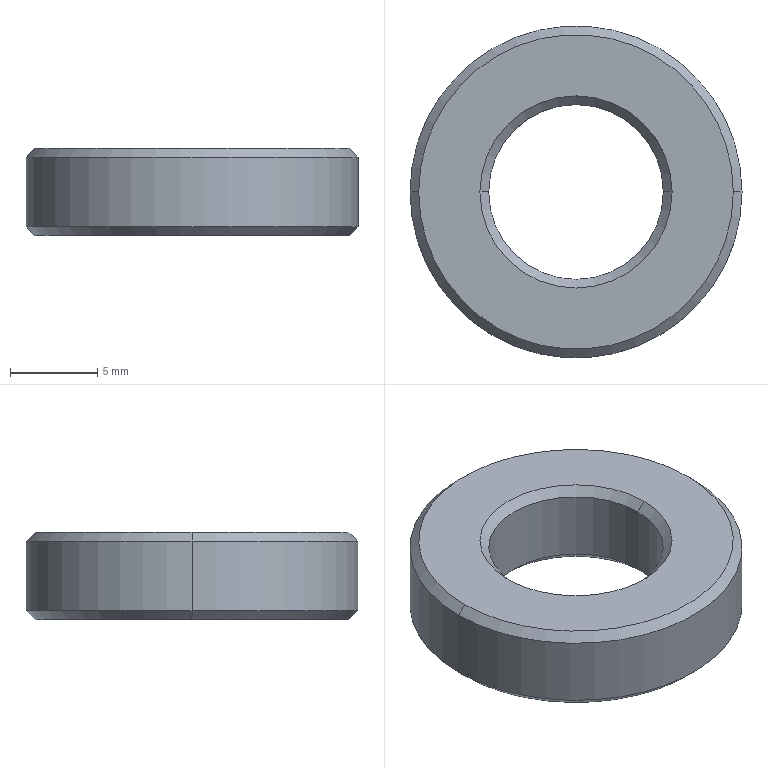Part | STEP file | deep groove bearing 6800 | 1 solid | 14 faces | box 19 x 19 x 5 mm | volume 1002 mm3 | cone 8 | cylinder 4 | plane 2 | commonest cylinder face diameters 10 x2 19 x2
STEP:
#1=CARTESIAN_POINT('',(0.,0.,0.));
#2=DIRECTION('',(0.,0.,1.));
#3=DIRECTION('',(1.,0.,0.));
#4=AXIS2_PLACEMENT_3D('',#1,#2,#3);
#5=CARTESIAN_POINT('',(9.,0.,5.));
#6=VERTEX_POINT('',#5);
#7=CARTESIAN_POINT('',(-9.,0.,5.));
#8=VERTEX_POINT('',#7);
#9=CARTESIAN_POINT('',(0.,0.,5.));
#10=DIRECTION('',(0.,0.,1.));
#11=DIRECTION('',(1.,0.,0.));
#12=AXIS2_PLACEMENT_3D('',#9,#10,#11);
#13=CIRCLE('',#12,9.);
#14=CARTESIAN_POINT('',(0.,0.,5.));
#15=DIRECTION('',(0.,0.,-1.));
#16=DIRECTION('',(-1.,0.,0.));
#17=AXIS2_PLACEMENT_3D('',#14,#15,#16);
#18=CONICAL_SURFACE('',#17,9.,0.7854);
#19=CARTESIAN_POINT('',(3.142,0.));
#20=DIRECTION('',(-1.,0.));
#21=VECTOR('',#20,1.);
#22=LINE('',#19,#21);
#23=(GEOMETRIC_REPRESENTATION_CONTEXT(2)PARAMETRIC_REPRESENTATION_CONTEXT()REPRESENTATION_CONTEXT('',''));
#24=DEFINITIONAL_REPRESENTATION('',(#22),#23);
#25=PCURVE('',#18,#24);
#26=CARTESIAN_POINT('',(0.,0.,5.));
#27=DIRECTION('',(0.,0.,1.));
#28=DIRECTION('',(1.,0.,0.));
#29=AXIS2_PLACEMENT_3D('',#26,#27,#28);
#30=PLANE('',#29);
#31=CARTESIAN_POINT('',(0.,0.));
#32=DIRECTION('',(1.,0.));
#33=AXIS2_PLACEMENT_2D('',#31,#32);
#34=CIRCLE('',#33,9.);
#35=(GEOMETRIC_REPRESENTATION_CONTEXT(2)PARAMETRIC_REPRESENTATION_CONTEXT()REPRESENTATION_CONTEXT('',''));
#36=DEFINITIONAL_REPRESENTATION('',(#34),#35);
#37=PCURVE('',#30,#36);
#38=SURFACE_CURVE('',#13,(#25,#37),.PCURVE_S1.);
#39=EDGE_CURVE('',#6,#8,#38,.T.);
#40=ORIENTED_EDGE('',*,*,#39,.F.);
#41=CARTESIAN_POINT('',(9.5,0.,4.5));
#42=VERTEX_POINT('',#41);
#43=CARTESIAN_POINT('',(9.,0.,5.));
#44=DIRECTION('',(0.7071,0.,-0.7071));
#45=VECTOR('',#44,1.);
#46=LINE('',#43,#45);
#47=CARTESIAN_POINT('',(3.142,0.));
#48=DIRECTION('',(0.,1.));
#49=VECTOR('',#48,1.);
#50=LINE('',#47,#49);
#51=(GEOMETRIC_REPRESENTATION_CONTEXT(2)PARAMETRIC_REPRESENTATION_CONTEXT()REPRESENTATION_CONTEXT('',''));
#52=DEFINITIONAL_REPRESENTATION('',(#50),#51);
#53=PCURVE('',#18,#52);
#54=CARTESIAN_POINT('',(0.,0.,5.));
#55=DIRECTION('',(0.,0.,-1.));
#56=DIRECTION('',(-1.,0.,0.));
#57=AXIS2_PLACEMENT_3D('',#54,#55,#56);
#58=CONICAL_SURFACE('',#57,9.,0.7854);
#59=CARTESIAN_POINT('',(3.142,0.));
#60=DIRECTION('',(0.,1.));
#61=VECTOR('',#60,1.);
#62=LINE('',#59,#61);
#63=(GEOMETRIC_REPRESENTATION_CONTEXT(2)PARAMETRIC_REPRESENTATION_CONTEXT()REPRESENTATION_CONTEXT('',''));
#64=DEFINITIONAL_REPRESENTATION('',(#62),#63);
#65=PCURVE('',#58,#64);
#66=SURFACE_CURVE('',#46,(#53,#65),.PCURVE_S1.);
#67=EDGE_CURVE('',#6,#42,#66,.T.);
#68=ORIENTED_EDGE('',*,*,#67,.T.);
#69=CARTESIAN_POINT('',(-9.5,0.,4.5));
#70=VERTEX_POINT('',#69);
#71=CARTESIAN_POINT('',(0.,0.,4.5));
#72=DIRECTION('',(0.,0.,-1.));
#73=DIRECTION('',(1.,0.,0.));
#74=AXIS2_PLACEMENT_3D('',#71,#72,#73);
#75=CIRCLE('',#74,9.5);
#76=CARTESIAN_POINT('',(-3.142,0.5));
#77=DIRECTION('',(1.,0.));
#78=VECTOR('',#77,1.);
#79=LINE('',#76,#78);
#80=(GEOMETRIC_REPRESENTATION_CONTEXT(2)PARAMETRIC_REPRESENTATION_CONTEXT()REPRESENTATION_CONTEXT('',''));
#81=DEFINITIONAL_REPRESENTATION('',(#79),#80);
#82=PCURVE('',#18,#81);
#83=CARTESIAN_POINT('',(0.,0.,5.));
#84=DIRECTION('',(0.,0.,-1.));
#85=DIRECTION('',(-1.,0.,0.));
#86=AXIS2_PLACEMENT_3D('',#83,#84,#85);
#87=CYLINDRICAL_SURFACE('',#86,9.5);
#88=CARTESIAN_POINT('',(-3.142,0.5));
#89=DIRECTION('',(1.,0.));
#90=VECTOR('',#89,1.);
#91=LINE('',#88,#90);
#92=(GEOMETRIC_REPRESENTATION_CONTEXT(2)PARAMETRIC_REPRESENTATION_CONTEXT()REPRESENTATION_CONTEXT('',''));
#93=DEFINITIONAL_REPRESENTATION('',(#91),#92);
#94=PCURVE('',#87,#93);
#95=SURFACE_CURVE('',#75,(#82,#94),.PCURVE_S1.);
#96=EDGE_CURVE('',#70,#42,#95,.T.);
#97=ORIENTED_EDGE('',*,*,#96,.F.);
#98=CARTESIAN_POINT('',(-9.,0.,5.));
#99=DIRECTION('',(-0.7071,0.,-0.7071));
#100=VECTOR('',#99,1.);
#101=LINE('',#98,#100);
#102=CARTESIAN_POINT('',(0.,0.));
#103=DIRECTION('',(0.,1.));
#104=VECTOR('',#103,1.);
#105=LINE('',#102,#104);
#106=(GEOMETRIC_REPRESENTATION_CONTEXT(2)PARAMETRIC_REPRESENTATION_CONTEXT()REPRESENTATION_CONTEXT('',''));
#107=DEFINITIONAL_REPRESENTATION('',(#105),#106);
#108=PCURVE('',#18,#107);
#109=CARTESIAN_POINT('',(6.283,0.));
#110=DIRECTION('',(0.,1.));
#111=VECTOR('',#110,1.);
#112=LINE('',#109,#111);
#113=(GEOMETRIC_REPRESENTATION_CONTEXT(2)PARAMETRIC_REPRESENTATION_CONTEXT()REPRESENTATION_CONTEXT('',''));
#114=DEFINITIONAL_REPRESENTATION('',(#112),#113);
#115=PCURVE('',#58,#114);
#116=SURFACE_CURVE('',#101,(#108,#115),.PCURVE_S1.);
#117=EDGE_CURVE('',#8,#70,#116,.T.);
#118=ORIENTED_EDGE('',*,*,#117,.F.);
#119=EDGE_LOOP('',(#40,#68,#97,#118));
#120=FACE_BOUND('',#119,.T.);
#121=ADVANCED_FACE('',(#120),#18,.T.);
#122=CARTESIAN_POINT('',(-9.,0.,0.));
#123=VERTEX_POINT('',#122);
#124=CARTESIAN_POINT('',(9.,0.,0.));
#125=VERTEX_POINT('',#124);
#126=CARTESIAN_POINT('',(0.,0.,0.));
#127=DIRECTION('',(0.,0.,-1.));
#128=DIRECTION('',(1.,0.,0.));
#129=AXIS2_PLACEMENT_3D('',#126,#127,#128);
#130=CIRCLE('',#129,9.);
#131=CARTESIAN_POINT('',(0.,0.,0.5));
#132=DIRECTION('',(0.,0.,1.));
#133=DIRECTION('',(1.,0.,0.));
#134=AXIS2_PLACEMENT_3D('',#131,#132,#133);
#135=CONICAL_SURFACE('',#134,9.5,0.7854);
#136=CARTESIAN_POINT('',(6.283,-0.5));
#137=DIRECTION('',(-1.,0.));
#138=VECTOR('',#137,1.);
#139=LINE('',#136,#138);
#140=(GEOMETRIC_REPRESENTATION_CONTEXT(2)PARAMETRIC_REPRESENTATION_CONTEXT()REPRESENTATION_CONTEXT('',''));
#141=DEFINITIONAL_REPRESENTATION('',(#139),#140);
#142=PCURVE('',#135,#141);
#143=CARTESIAN_POINT('',(0.,0.,0.));
#144=DIRECTION('',(0.,0.,1.));
#145=DIRECTION('',(1.,0.,0.));
#146=AXIS2_PLACEMENT_3D('',#143,#144,#145);
#147=PLANE('',#146);
#148=CARTESIAN_POINT('',(9.,0.));
#149=CARTESIAN_POINT('',(9.,-15.588));
#150=CARTESIAN_POINT('',(-4.5,-7.794));
#151=CARTESIAN_POINT('',(-18.,0.));
#152=CARTESIAN_POINT('',(-4.5,7.794));
#153=CARTESIAN_POINT('',(9.,15.588));
#154=CARTESIAN_POINT('',(9.,0.));
#155=(BOUNDED_CURVE()B_SPLINE_CURVE(2,(#148,#149,#150,#151,#152,#153,#154),.UNSPECIFIED.,.T.,.F.)B_SPLINE_CURVE_WITH_KNOTS((1,2,2,2,2,1),(-2.094,0.,2.094,4.189,6.283,8.378),.UNSPECIFIED.)CURVE()GEOMETRIC_REPRESENTATION_ITEM()RATIONAL_B_SPLINE_CURVE((1.,0.5,1.,0.5,1.,0.5,1.))REPRESENTATION_ITEM(''));
#156=(GEOMETRIC_REPRESENTATION_CONTEXT(2)PARAMETRIC_REPRESENTATION_CONTEXT()REPRESENTATION_CONTEXT('',''));
#157=DEFINITIONAL_REPRESENTATION('',(#155),#156);
#158=PCURVE('',#147,#157);
#159=SURFACE_CURVE('',#130,(#142,#158),.PCURVE_S1.);
#160=EDGE_CURVE('',#123,#125,#159,.T.);
#161=ORIENTED_EDGE('',*,*,#160,.F.);
#162=CARTESIAN_POINT('',(-9.5,0.,0.5));
#163=VERTEX_POINT('',#162);
#164=CARTESIAN_POINT('',(-9.5,0.,0.5));
#165=DIRECTION('',(-0.7071,0.,0.7071));
#166=VECTOR('',#165,1.);
#167=LINE('',#164,#166);
#168=CARTESIAN_POINT('',(3.142,0.));
#169=DIRECTION('',(0.,1.));
#170=VECTOR('',#169,1.);
#171=LINE('',#168,#170);
#172=(GEOMETRIC_REPRESENTATION_CONTEXT(2)PARAMETRIC_REPRESENTATION_CONTEXT()REPRESENTATION_CONTEXT('',''));
#173=DEFINITIONAL_REPRESENTATION('',(#171),#172);
#174=PCURVE('',#135,#173);
#175=CARTESIAN_POINT('',(0.,0.,0.5));
#176=DIRECTION('',(0.,0.,1.));
#177=DIRECTION('',(1.,0.,0.));
#178=AXIS2_PLACEMENT_3D('',#175,#176,#177);
#179=CONICAL_SURFACE('',#178,9.5,0.7854);
#180=CARTESIAN_POINT('',(3.142,0.));
#181=DIRECTION('',(0.,1.));
#182=VECTOR('',#181,1.);
#183=LINE('',#180,#182);
#184=(GEOMETRIC_REPRESENTATION_CONTEXT(2)PARAMETRIC_REPRESENTATION_CONTEXT()REPRESENTATION_CONTEXT('',''));
#185=DEFINITIONAL_REPRESENTATION('',(#183),#184);
#186=PCURVE('',#179,#185);
#187=SURFACE_CURVE('',#167,(#174,#186),.PCURVE_S1.);
#188=EDGE_CURVE('',#123,#163,#187,.T.);
#189=ORIENTED_EDGE('',*,*,#188,.T.);
#190=CARTESIAN_POINT('',(9.5,0.,0.5));
#191=VERTEX_POINT('',#190);
#192=CARTESIAN_POINT('',(0.,0.,0.5));
#193=DIRECTION('',(0.,0.,1.));
#194=DIRECTION('',(1.,0.,0.));
#195=AXIS2_PLACEMENT_3D('',#192,#193,#194);
#196=CIRCLE('',#195,9.5);
#197=CARTESIAN_POINT('',(0.,0.));
#198=DIRECTION('',(1.,0.));
#199=VECTOR('',#198,1.);
#200=LINE('',#197,#199);
#201=(GEOMETRIC_REPRESENTATION_CONTEXT(2)PARAMETRIC_REPRESENTATION_CONTEXT()REPRESENTATION_CONTEXT('',''));
#202=DEFINITIONAL_REPRESENTATION('',(#200),#201);
#203=PCURVE('',#135,#202);
#204=CARTESIAN_POINT('',(3.142,4.5));
#205=DIRECTION('',(-1.,0.));
#206=VECTOR('',#205,1.);
#207=LINE('',#204,#206);
#208=(GEOMETRIC_REPRESENTATION_CONTEXT(2)PARAMETRIC_REPRESENTATION_CONTEXT()REPRESENTATION_CONTEXT('',''));
#209=DEFINITIONAL_REPRESENTATION('',(#207),#208);
#210=PCURVE('',#87,#209);
#211=SURFACE_CURVE('',#196,(#203,#210),.PCURVE_S1.);
#212=EDGE_CURVE('',#191,#163,#211,.T.);
#213=ORIENTED_EDGE('',*,*,#212,.F.);
#214=CARTESIAN_POINT('',(9.5,0.,0.5));
#215=DIRECTION('',(0.7071,0.,0.7071));
#216=VECTOR('',#215,1.);
#217=LINE('',#214,#216);
#218=CARTESIAN_POINT('',(0.,0.));
#219=DIRECTION('',(0.,1.));
#220=VECTOR('',#219,1.);
#221=LINE('',#218,#220);
#222=(GEOMETRIC_REPRESENTATION_CONTEXT(2)PARAMETRIC_REPRESENTATION_CONTEXT()REPRESENTATION_CONTEXT('',''));
#223=DEFINITIONAL_REPRESENTATION('',(#221),#222);
#224=PCURVE('',#135,#223);
#225=CARTESIAN_POINT('',(6.283,0.));
#226=DIRECTION('',(0.,1.));
#227=VECTOR('',#226,1.);
#228=LINE('',#225,#227);
#229=(GEOMETRIC_REPRESENTATION_CONTEXT(2)PARAMETRIC_REPRESENTATION_CONTEXT()REPRESENTATION_CONTEXT('',''));
#230=DEFINITIONAL_REPRESENTATION('',(#228),#229);
#231=PCURVE('',#179,#230);
#232=SURFACE_CURVE('',#217,(#224,#231),.PCURVE_S1.);
#233=EDGE_CURVE('',#125,#191,#232,.T.);
#234=ORIENTED_EDGE('',*,*,#233,.F.);
#235=EDGE_LOOP('',(#161,#189,#213,#234));
#236=FACE_BOUND('',#235,.T.);
#237=ADVANCED_FACE('',(#236),#135,.T.);
#238=CARTESIAN_POINT('',(5.,0.,4.5));
#239=VERTEX_POINT('',#238);
#240=CARTESIAN_POINT('',(5.5,0.,5.));
#241=VERTEX_POINT('',#240);
#242=CARTESIAN_POINT('',(5.,0.,4.5));
#243=DIRECTION('',(0.7071,0.,0.7071));
#244=VECTOR('',#243,1.);
#245=LINE('',#242,#244);
#246=CARTESIAN_POINT('',(0.,0.,4.5));
#247=DIRECTION('',(0.,0.,1.));
#248=DIRECTION('',(1.,0.,0.));
#249=AXIS2_PLACEMENT_3D('',#246,#247,#248);
#250=CONICAL_SURFACE('',#249,5.,0.7854);
#251=CARTESIAN_POINT('',(6.283,0.));
#252=DIRECTION('',(0.,1.));
#253=VECTOR('',#252,1.);
#254=LINE('',#251,#253);
#255=(GEOMETRIC_REPRESENTATION_CONTEXT(2)PARAMETRIC_REPRESENTATION_CONTEXT()REPRESENTATION_CONTEXT('',''));
#256=DEFINITIONAL_REPRESENTATION('',(#254),#255);
#257=PCURVE('',#250,#256);
#258=CARTESIAN_POINT('',(0.,0.,4.5));
#259=DIRECTION('',(0.,0.,1.));
#260=DIRECTION('',(1.,0.,0.));
#261=AXIS2_PLACEMENT_3D('',#258,#259,#260);
#262=CONICAL_SURFACE('',#261,5.,0.7854);
#263=CARTESIAN_POINT('',(0.,0.));
#264=DIRECTION('',(0.,1.));
#265=VECTOR('',#264,1.);
#266=LINE('',#263,#265);
#267=(GEOMETRIC_REPRESENTATION_CONTEXT(2)PARAMETRIC_REPRESENTATION_CONTEXT()REPRESENTATION_CONTEXT('',''));
#268=DEFINITIONAL_REPRESENTATION('',(#266),#267);
#269=PCURVE('',#262,#268);
#270=SURFACE_CURVE('',#245,(#257,#269),.PCURVE_S1.);
#271=EDGE_CURVE('',#239,#241,#270,.T.);
#272=ORIENTED_EDGE('',*,*,#271,.T.);
#273=CARTESIAN_POINT('',(-5.5,0.,5.));
#274=VERTEX_POINT('',#273);
#275=CARTESIAN_POINT('',(0.,0.,5.));
#276=DIRECTION('',(0.,0.,-1.));
#277=DIRECTION('',(1.,0.,0.));
#278=AXIS2_PLACEMENT_3D('',#275,#276,#277);
#279=CIRCLE('',#278,5.5);
#280=CARTESIAN_POINT('',(6.283,0.5));
#281=DIRECTION('',(-1.,0.));
#282=VECTOR('',#281,1.);
#283=LINE('',#280,#282);
#284=(GEOMETRIC_REPRESENTATION_CONTEXT(2)PARAMETRIC_REPRESENTATION_CONTEXT()REPRESENTATION_CONTEXT('',''));
#285=DEFINITIONAL_REPRESENTATION('',(#283),#284);
#286=PCURVE('',#250,#285);
#287=CARTESIAN_POINT('',(5.5,0.));
#288=CARTESIAN_POINT('',(5.5,-9.526));
#289=CARTESIAN_POINT('',(-2.75,-4.763));
#290=CARTESIAN_POINT('',(-11.,0.));
#291=CARTESIAN_POINT('',(-2.75,4.763));
#292=CARTESIAN_POINT('',(5.5,9.526));
#293=CARTESIAN_POINT('',(5.5,0.));
#294=(BOUNDED_CURVE()B_SPLINE_CURVE(2,(#287,#288,#289,#290,#291,#292,#293),.UNSPECIFIED.,.T.,.F.)B_SPLINE_CURVE_WITH_KNOTS((1,2,2,2,2,1),(-2.094,0.,2.094,4.189,6.283,8.378),.UNSPECIFIED.)CURVE()GEOMETRIC_REPRESENTATION_ITEM()RATIONAL_B_SPLINE_CURVE((1.,0.5,1.,0.5,1.,0.5,1.))REPRESENTATION_ITEM(''));
#295=(GEOMETRIC_REPRESENTATION_CONTEXT(2)PARAMETRIC_REPRESENTATION_CONTEXT()REPRESENTATION_CONTEXT('',''));
#296=DEFINITIONAL_REPRESENTATION('',(#294),#295);
#297=PCURVE('',#30,#296);
#298=SURFACE_CURVE('',#279,(#286,#297),.PCURVE_S1.);
#299=EDGE_CURVE('',#241,#274,#298,.T.);
#300=ORIENTED_EDGE('',*,*,#299,.T.);
#301=CARTESIAN_POINT('',(-5.,0.,4.5));
#302=VERTEX_POINT('',#301);
#303=CARTESIAN_POINT('',(-5.,0.,4.5));
#304=DIRECTION('',(-0.7071,0.,0.7071));
#305=VECTOR('',#304,1.);
#306=LINE('',#303,#305);
#307=CARTESIAN_POINT('',(3.142,0.));
#308=DIRECTION('',(0.,1.));
#309=VECTOR('',#308,1.);
#310=LINE('',#307,#309);
#311=(GEOMETRIC_REPRESENTATION_CONTEXT(2)PARAMETRIC_REPRESENTATION_CONTEXT()REPRESENTATION_CONTEXT('',''));
#312=DEFINITIONAL_REPRESENTATION('',(#310),#311);
#313=PCURVE('',#250,#312);
#314=CARTESIAN_POINT('',(3.142,0.));
#315=DIRECTION('',(0.,1.));
#316=VECTOR('',#315,1.);
#317=LINE('',#314,#316);
#318=(GEOMETRIC_REPRESENTATION_CONTEXT(2)PARAMETRIC_REPRESENTATION_CONTEXT()REPRESENTATION_CONTEXT('',''));
#319=DEFINITIONAL_REPRESENTATION('',(#317),#318);
#320=PCURVE('',#262,#319);
#321=SURFACE_CURVE('',#306,(#313,#320),.PCURVE_S1.);
#322=EDGE_CURVE('',#302,#274,#321,.T.);
#323=ORIENTED_EDGE('',*,*,#322,.F.);
#324=CARTESIAN_POINT('',(0.,0.,4.5));
#325=DIRECTION('',(0.,0.,1.));
#326=DIRECTION('',(1.,0.,0.));
#327=AXIS2_PLACEMENT_3D('',#324,#325,#326);
#328=CIRCLE('',#327,5.);
#329=CARTESIAN_POINT('',(0.,0.));
#330=DIRECTION('',(1.,0.));
#331=VECTOR('',#330,1.);
#332=LINE('',#329,#331);
#333=(GEOMETRIC_REPRESENTATION_CONTEXT(2)PARAMETRIC_REPRESENTATION_CONTEXT()REPRESENTATION_CONTEXT('',''));
#334=DEFINITIONAL_REPRESENTATION('',(#332),#333);
#335=PCURVE('',#250,#334);
#336=CARTESIAN_POINT('',(0.,0.,5.));
#337=DIRECTION('',(0.,0.,-1.));
#338=DIRECTION('',(-1.,0.,0.));
#339=AXIS2_PLACEMENT_3D('',#336,#337,#338);
#340=CYLINDRICAL_SURFACE('',#339,5.);
#341=CARTESIAN_POINT('',(9.425,0.5));
#342=DIRECTION('',(-1.,0.));
#343=VECTOR('',#342,1.);
#344=LINE('',#341,#343);
#345=(GEOMETRIC_REPRESENTATION_CONTEXT(2)PARAMETRIC_REPRESENTATION_CONTEXT()REPRESENTATION_CONTEXT('',''));
#346=DEFINITIONAL_REPRESENTATION('',(#344),#345);
#347=PCURVE('',#340,#346);
#348=SURFACE_CURVE('',#328,(#335,#347),.PCURVE_S1.);
#349=EDGE_CURVE('',#302,#239,#348,.T.);
#350=ORIENTED_EDGE('',*,*,#349,.T.);
#351=EDGE_LOOP('',(#272,#300,#323,#350));
#352=FACE_BOUND('',#351,.F.);
#353=ADVANCED_FACE('',(#352),#250,.F.);
#354=CARTESIAN_POINT('',(-5.,0.,0.5));
#355=VERTEX_POINT('',#354);
#356=CARTESIAN_POINT('',(-5.5,0.,0.));
#357=VERTEX_POINT('',#356);
#358=CARTESIAN_POINT('',(-5.5,0.,0.));
#359=DIRECTION('',(-0.7071,0.,-0.7071));
#360=VECTOR('',#359,1.);
#361=LINE('',#358,#360);
#362=CARTESIAN_POINT('',(0.,0.,0.));
#363=DIRECTION('',(0.,0.,-1.));
#364=DIRECTION('',(-1.,0.,0.));
#365=AXIS2_PLACEMENT_3D('',#362,#363,#364);
#366=CONICAL_SURFACE('',#365,5.5,0.7854);
#367=CARTESIAN_POINT('',(6.283,0.));
#368=DIRECTION('',(0.,1.));
#369=VECTOR('',#368,1.);
#370=LINE('',#367,#369);
#371=(GEOMETRIC_REPRESENTATION_CONTEXT(2)PARAMETRIC_REPRESENTATION_CONTEXT()REPRESENTATION_CONTEXT('',''));
#372=DEFINITIONAL_REPRESENTATION('',(#370),#371);
#373=PCURVE('',#366,#372);
#374=CARTESIAN_POINT('',(0.,0.,0.));
#375=DIRECTION('',(0.,0.,-1.));
#376=DIRECTION('',(-1.,0.,0.));
#377=AXIS2_PLACEMENT_3D('',#374,#375,#376);
#378=CONICAL_SURFACE('',#377,5.5,0.7854);
#379=CARTESIAN_POINT('',(0.,0.));
#380=DIRECTION('',(0.,1.));
#381=VECTOR('',#380,1.);
#382=LINE('',#379,#381);
#383=(GEOMETRIC_REPRESENTATION_CONTEXT(2)PARAMETRIC_REPRESENTATION_CONTEXT()REPRESENTATION_CONTEXT('',''));
#384=DEFINITIONAL_REPRESENTATION('',(#382),#383);
#385=PCURVE('',#378,#384);
#386=SURFACE_CURVE('',#361,(#373,#385),.PCURVE_S1.);
#387=EDGE_CURVE('',#355,#357,#386,.T.);
#388=ORIENTED_EDGE('',*,*,#387,.T.);
#389=CARTESIAN_POINT('',(5.5,0.,0.));
#390=VERTEX_POINT('',#389);
#391=CARTESIAN_POINT('',(0.,0.,0.));
#392=DIRECTION('',(0.,0.,1.));
#393=DIRECTION('',(1.,0.,0.));
#394=AXIS2_PLACEMENT_3D('',#391,#392,#393);
#395=CIRCLE('',#394,5.5);
#396=CARTESIAN_POINT('',(9.425,0.));
#397=DIRECTION('',(-1.,0.));
#398=VECTOR('',#397,1.);
#399=LINE('',#396,#398);
#400=(GEOMETRIC_REPRESENTATION_CONTEXT(2)PARAMETRIC_REPRESENTATION_CONTEXT()REPRESENTATION_CONTEXT('',''));
#401=DEFINITIONAL_REPRESENTATION('',(#399),#400);
#402=PCURVE('',#366,#401);
#403=CARTESIAN_POINT('',(0.,0.));
#404=DIRECTION('',(1.,0.));
#405=AXIS2_PLACEMENT_2D('',#403,#404);
#406=CIRCLE('',#405,5.5);
#407=(GEOMETRIC_REPRESENTATION_CONTEXT(2)PARAMETRIC_REPRESENTATION_CONTEXT()REPRESENTATION_CONTEXT('',''));
#408=DEFINITIONAL_REPRESENTATION('',(#406),#407);
#409=PCURVE('',#147,#408);
#410=SURFACE_CURVE('',#395,(#402,#409),.PCURVE_S1.);
#411=EDGE_CURVE('',#357,#390,#410,.T.);
#412=ORIENTED_EDGE('',*,*,#411,.T.);
#413=CARTESIAN_POINT('',(5.,0.,0.5));
#414=VERTEX_POINT('',#413);
#415=CARTESIAN_POINT('',(5.5,0.,0.));
#416=DIRECTION('',(0.7071,0.,-0.7071));
#417=VECTOR('',#416,1.);
#418=LINE('',#415,#417);
#419=CARTESIAN_POINT('',(3.142,0.));
#420=DIRECTION('',(0.,1.));
#421=VECTOR('',#420,1.);
#422=LINE('',#419,#421);
#423=(GEOMETRIC_REPRESENTATION_CONTEXT(2)PARAMETRIC_REPRESENTATION_CONTEXT()REPRESENTATION_CONTEXT('',''));
#424=DEFINITIONAL_REPRESENTATION('',(#422),#423);
#425=PCURVE('',#366,#424);
#426=CARTESIAN_POINT('',(3.142,0.));
#427=DIRECTION('',(0.,1.));
#428=VECTOR('',#427,1.);
#429=LINE('',#426,#428);
#430=(GEOMETRIC_REPRESENTATION_CONTEXT(2)PARAMETRIC_REPRESENTATION_CONTEXT()REPRESENTATION_CONTEXT('',''));
#431=DEFINITIONAL_REPRESENTATION('',(#429),#430);
#432=PCURVE('',#378,#431);
#433=SURFACE_CURVE('',#418,(#425,#432),.PCURVE_S1.);
#434=EDGE_CURVE('',#414,#390,#433,.T.);
#435=ORIENTED_EDGE('',*,*,#434,.F.);
#436=CARTESIAN_POINT('',(0.,0.,0.5));
#437=DIRECTION('',(0.,0.,-1.));
#438=DIRECTION('',(1.,0.,0.));
#439=AXIS2_PLACEMENT_3D('',#436,#437,#438);
#440=CIRCLE('',#439,5.);
#441=CARTESIAN_POINT('',(3.142,-0.5));
#442=DIRECTION('',(1.,0.));
#443=VECTOR('',#442,1.);
#444=LINE('',#441,#443);
#445=(GEOMETRIC_REPRESENTATION_CONTEXT(2)PARAMETRIC_REPRESENTATION_CONTEXT()REPRESENTATION_CONTEXT('',''));
#446=DEFINITIONAL_REPRESENTATION('',(#444),#445);
#447=PCURVE('',#366,#446);
#448=CARTESIAN_POINT('',(3.142,4.5));
#449=DIRECTION('',(1.,0.));
#450=VECTOR('',#449,1.);
#451=LINE('',#448,#450);
#452=(GEOMETRIC_REPRESENTATION_CONTEXT(2)PARAMETRIC_REPRESENTATION_CONTEXT()REPRESENTATION_CONTEXT('',''));
#453=DEFINITIONAL_REPRESENTATION('',(#451),#452);
#454=PCURVE('',#340,#453);
#455=SURFACE_CURVE('',#440,(#447,#454),.PCURVE_S1.);
#456=EDGE_CURVE('',#414,#355,#455,.T.);
#457=ORIENTED_EDGE('',*,*,#456,.T.);
#458=EDGE_LOOP('',(#388,#412,#435,#457));
#459=FACE_BOUND('',#458,.F.);
#460=ADVANCED_FACE('',(#459),#366,.F.);
#461=CARTESIAN_POINT('',(-5.,0.,5.));
#462=DIRECTION('',(0.,0.,-1.));
#463=VECTOR('',#462,1.);
#464=LINE('',#461,#463);
#465=CARTESIAN_POINT('',(6.283,0.));
#466=DIRECTION('',(0.,1.));
#467=VECTOR('',#466,1.);
#468=LINE('',#465,#467);
#469=(GEOMETRIC_REPRESENTATION_CONTEXT(2)PARAMETRIC_REPRESENTATION_CONTEXT()REPRESENTATION_CONTEXT('',''));
#470=DEFINITIONAL_REPRESENTATION('',(#468),#469);
#471=PCURVE('',#340,#470);
#472=CARTESIAN_POINT('',(0.,0.,5.));
#473=DIRECTION('',(0.,0.,-1.));
#474=DIRECTION('',(-1.,0.,0.));
#475=AXIS2_PLACEMENT_3D('',#472,#473,#474);
#476=CYLINDRICAL_SURFACE('',#475,5.);
#477=CARTESIAN_POINT('',(0.,0.));
#478=DIRECTION('',(0.,1.));
#479=VECTOR('',#478,1.);
#480=LINE('',#477,#479);
#481=(GEOMETRIC_REPRESENTATION_CONTEXT(2)PARAMETRIC_REPRESENTATION_CONTEXT()REPRESENTATION_CONTEXT('',''));
#482=DEFINITIONAL_REPRESENTATION('',(#480),#481);
#483=PCURVE('',#476,#482);
#484=SURFACE_CURVE('',#464,(#471,#483),.PCURVE_S1.);
#485=EDGE_CURVE('',#302,#355,#484,.T.);
#486=ORIENTED_EDGE('',*,*,#485,.T.);
#487=ORIENTED_EDGE('',*,*,#456,.F.);
#488=CARTESIAN_POINT('',(5.,0.,5.));
#489=DIRECTION('',(0.,0.,-1.));
#490=VECTOR('',#489,1.);
#491=LINE('',#488,#490);
#492=CARTESIAN_POINT('',(3.142,0.));
#493=DIRECTION('',(0.,1.));
#494=VECTOR('',#493,1.);
#495=LINE('',#492,#494);
#496=(GEOMETRIC_REPRESENTATION_CONTEXT(2)PARAMETRIC_REPRESENTATION_CONTEXT()REPRESENTATION_CONTEXT('',''));
#497=DEFINITIONAL_REPRESENTATION('',(#495),#496);
#498=PCURVE('',#340,#497);
#499=CARTESIAN_POINT('',(3.142,0.));
#500=DIRECTION('',(0.,1.));
#501=VECTOR('',#500,1.);
#502=LINE('',#499,#501);
#503=(GEOMETRIC_REPRESENTATION_CONTEXT(2)PARAMETRIC_REPRESENTATION_CONTEXT()REPRESENTATION_CONTEXT('',''));
#504=DEFINITIONAL_REPRESENTATION('',(#502),#503);
#505=PCURVE('',#476,#504);
#506=SURFACE_CURVE('',#491,(#498,#505),.PCURVE_S1.);
#507=EDGE_CURVE('',#239,#414,#506,.T.);
#508=ORIENTED_EDGE('',*,*,#507,.F.);
#509=ORIENTED_EDGE('',*,*,#349,.F.);
#510=EDGE_LOOP('',(#486,#487,#508,#509));
#511=FACE_BOUND('',#510,.F.);
#512=ADVANCED_FACE('',(#511),#340,.F.);
#513=ORIENTED_EDGE('',*,*,#96,.T.);
#514=CARTESIAN_POINT('',(9.5,0.,5.));
#515=DIRECTION('',(0.,0.,-1.));
#516=VECTOR('',#515,1.);
#517=LINE('',#514,#516);
#518=CARTESIAN_POINT('',(3.142,0.));
#519=DIRECTION('',(0.,1.));
#520=VECTOR('',#519,1.);
#521=LINE('',#518,#520);
#522=(GEOMETRIC_REPRESENTATION_CONTEXT(2)PARAMETRIC_REPRESENTATION_CONTEXT()REPRESENTATION_CONTEXT('',''));
#523=DEFINITIONAL_REPRESENTATION('',(#521),#522);
#524=PCURVE('',#87,#523);
#525=CARTESIAN_POINT('',(0.,0.,5.));
#526=DIRECTION('',(0.,0.,-1.));
#527=DIRECTION('',(-1.,0.,0.));
#528=AXIS2_PLACEMENT_3D('',#525,#526,#527);
#529=CYLINDRICAL_SURFACE('',#528,9.5);
#530=CARTESIAN_POINT('',(3.142,0.));
#531=DIRECTION('',(0.,1.));
#532=VECTOR('',#531,1.);
#533=LINE('',#530,#532);
#534=(GEOMETRIC_REPRESENTATION_CONTEXT(2)PARAMETRIC_REPRESENTATION_CONTEXT()REPRESENTATION_CONTEXT('',''));
#535=DEFINITIONAL_REPRESENTATION('',(#533),#534);
#536=PCURVE('',#529,#535);
#537=SURFACE_CURVE('',#517,(#524,#536),.PCURVE_S1.);
#538=EDGE_CURVE('',#42,#191,#537,.T.);
#539=ORIENTED_EDGE('',*,*,#538,.T.);
#540=ORIENTED_EDGE('',*,*,#212,.T.);
#541=CARTESIAN_POINT('',(-9.5,0.,5.));
#542=DIRECTION('',(0.,0.,-1.));
#543=VECTOR('',#542,1.);
#544=LINE('',#541,#543);
#545=CARTESIAN_POINT('',(0.,0.));
#546=DIRECTION('',(0.,1.));
#547=VECTOR('',#546,1.);
#548=LINE('',#545,#547);
#549=(GEOMETRIC_REPRESENTATION_CONTEXT(2)PARAMETRIC_REPRESENTATION_CONTEXT()REPRESENTATION_CONTEXT('',''));
#550=DEFINITIONAL_REPRESENTATION('',(#548),#549);
#551=PCURVE('',#87,#550);
#552=CARTESIAN_POINT('',(6.283,0.));
#553=DIRECTION('',(0.,1.));
#554=VECTOR('',#553,1.);
#555=LINE('',#552,#554);
#556=(GEOMETRIC_REPRESENTATION_CONTEXT(2)PARAMETRIC_REPRESENTATION_CONTEXT()REPRESENTATION_CONTEXT('',''));
#557=DEFINITIONAL_REPRESENTATION('',(#555),#556);
#558=PCURVE('',#529,#557);
#559=SURFACE_CURVE('',#544,(#551,#558),.PCURVE_S1.);
#560=EDGE_CURVE('',#70,#163,#559,.T.);
#561=ORIENTED_EDGE('',*,*,#560,.F.);
#562=EDGE_LOOP('',(#513,#539,#540,#561));
#563=FACE_BOUND('',#562,.T.);
#564=ADVANCED_FACE('',(#563),#87,.T.);
#565=ORIENTED_EDGE('',*,*,#299,.T.);
#566=CARTESIAN_POINT('',(0.,0.,5.));
#567=DIRECTION('',(0.,0.,-1.));
#568=DIRECTION('',(1.,0.,0.));
#569=AXIS2_PLACEMENT_3D('',#566,#567,#568);
#570=CIRCLE('',#569,5.5);
#571=CARTESIAN_POINT('',(5.5,0.));
#572=CARTESIAN_POINT('',(5.5,-9.526));
#573=CARTESIAN_POINT('',(-2.75,-4.763));
#574=CARTESIAN_POINT('',(-11.,0.));
#575=CARTESIAN_POINT('',(-2.75,4.763));
#576=CARTESIAN_POINT('',(5.5,9.526));
#577=CARTESIAN_POINT('',(5.5,0.));
#578=(BOUNDED_CURVE()B_SPLINE_CURVE(2,(#571,#572,#573,#574,#575,#576,#577),.UNSPECIFIED.,.T.,.F.)B_SPLINE_CURVE_WITH_KNOTS((1,2,2,2,2,1),(-2.094,0.,2.094,4.189,6.283,8.378),.UNSPECIFIED.)CURVE()GEOMETRIC_REPRESENTATION_ITEM()RATIONAL_B_SPLINE_CURVE((1.,0.5,1.,0.5,1.,0.5,1.))REPRESENTATION_ITEM(''));
#579=(GEOMETRIC_REPRESENTATION_CONTEXT(2)PARAMETRIC_REPRESENTATION_CONTEXT()REPRESENTATION_CONTEXT('',''));
#580=DEFINITIONAL_REPRESENTATION('',(#578),#579);
#581=PCURVE('',#30,#580);
#582=CARTESIAN_POINT('',(6.283,0.5));
#583=DIRECTION('',(-1.,0.));
#584=VECTOR('',#583,1.);
#585=LINE('',#582,#584);
#586=(GEOMETRIC_REPRESENTATION_CONTEXT(2)PARAMETRIC_REPRESENTATION_CONTEXT()REPRESENTATION_CONTEXT('',''));
#587=DEFINITIONAL_REPRESENTATION('',(#585),#586);
#588=PCURVE('',#262,#587);
#589=SURFACE_CURVE('',#570,(#581,#588),.PCURVE_S1.);
#590=EDGE_CURVE('',#274,#241,#589,.T.);
#591=ORIENTED_EDGE('',*,*,#590,.T.);
#592=EDGE_LOOP('',(#565,#591));
#593=FACE_BOUND('',#592,.T.);
#594=CARTESIAN_POINT('',(0.,0.,5.));
#595=DIRECTION('',(0.,0.,1.));
#596=DIRECTION('',(1.,0.,0.));
#597=AXIS2_PLACEMENT_3D('',#594,#595,#596);
#598=CIRCLE('',#597,9.);
#599=CARTESIAN_POINT('',(0.,0.));
#600=DIRECTION('',(1.,0.));
#601=AXIS2_PLACEMENT_2D('',#599,#600);
#602=CIRCLE('',#601,9.);
#603=(GEOMETRIC_REPRESENTATION_CONTEXT(2)PARAMETRIC_REPRESENTATION_CONTEXT()REPRESENTATION_CONTEXT('',''));
#604=DEFINITIONAL_REPRESENTATION('',(#602),#603);
#605=PCURVE('',#30,#604);
#606=CARTESIAN_POINT('',(9.425,0.));
#607=DIRECTION('',(-1.,0.));
#608=VECTOR('',#607,1.);
#609=LINE('',#606,#608);
#610=(GEOMETRIC_REPRESENTATION_CONTEXT(2)PARAMETRIC_REPRESENTATION_CONTEXT()REPRESENTATION_CONTEXT('',''));
#611=DEFINITIONAL_REPRESENTATION('',(#609),#610);
#612=PCURVE('',#58,#611);
#613=SURFACE_CURVE('',#598,(#605,#612),.PCURVE_S1.);
#614=EDGE_CURVE('',#8,#6,#613,.T.);
#615=ORIENTED_EDGE('',*,*,#614,.T.);
#616=ORIENTED_EDGE('',*,*,#39,.T.);
#617=EDGE_LOOP('',(#615,#616));
#618=FACE_BOUND('',#617,.T.);
#619=ADVANCED_FACE('',(#593,#618),#30,.T.);
#620=ORIENTED_EDGE('',*,*,#411,.T.);
#621=CARTESIAN_POINT('',(0.,0.,0.));
#622=DIRECTION('',(0.,0.,1.));
#623=DIRECTION('',(1.,0.,0.));
#624=AXIS2_PLACEMENT_3D('',#621,#622,#623);
#625=CIRCLE('',#624,5.5);
#626=CARTESIAN_POINT('',(0.,0.));
#627=DIRECTION('',(1.,0.));
#628=AXIS2_PLACEMENT_2D('',#626,#627);
#629=CIRCLE('',#628,5.5);
#630=(GEOMETRIC_REPRESENTATION_CONTEXT(2)PARAMETRIC_REPRESENTATION_CONTEXT()REPRESENTATION_CONTEXT('',''));
#631=DEFINITIONAL_REPRESENTATION('',(#629),#630);
#632=PCURVE('',#147,#631);
#633=CARTESIAN_POINT('',(3.142,0.));
#634=DIRECTION('',(-1.,0.));
#635=VECTOR('',#634,1.);
#636=LINE('',#633,#635);
#637=(GEOMETRIC_REPRESENTATION_CONTEXT(2)PARAMETRIC_REPRESENTATION_CONTEXT()REPRESENTATION_CONTEXT('',''));
#638=DEFINITIONAL_REPRESENTATION('',(#636),#637);
#639=PCURVE('',#378,#638);
#640=SURFACE_CURVE('',#625,(#632,#639),.PCURVE_S1.);
#641=EDGE_CURVE('',#390,#357,#640,.T.);
#642=ORIENTED_EDGE('',*,*,#641,.T.);
#643=EDGE_LOOP('',(#620,#642));
#644=FACE_BOUND('',#643,.T.);
#645=CARTESIAN_POINT('',(0.,0.,0.));
#646=DIRECTION('',(0.,0.,-1.));
#647=DIRECTION('',(1.,0.,0.));
#648=AXIS2_PLACEMENT_3D('',#645,#646,#647);
#649=CIRCLE('',#648,9.);
#650=CARTESIAN_POINT('',(9.,0.));
#651=CARTESIAN_POINT('',(9.,-15.588));
#652=CARTESIAN_POINT('',(-4.5,-7.794));
#653=CARTESIAN_POINT('',(-18.,0.));
#654=CARTESIAN_POINT('',(-4.5,7.794));
#655=CARTESIAN_POINT('',(9.,15.588));
#656=CARTESIAN_POINT('',(9.,0.));
#657=(BOUNDED_CURVE()B_SPLINE_CURVE(2,(#650,#651,#652,#653,#654,#655,#656),.UNSPECIFIED.,.T.,.F.)B_SPLINE_CURVE_WITH_KNOTS((1,2,2,2,2,1),(-2.094,0.,2.094,4.189,6.283,8.378),.UNSPECIFIED.)CURVE()GEOMETRIC_REPRESENTATION_ITEM()RATIONAL_B_SPLINE_CURVE((1.,0.5,1.,0.5,1.,0.5,1.))REPRESENTATION_ITEM(''));
#658=(GEOMETRIC_REPRESENTATION_CONTEXT(2)PARAMETRIC_REPRESENTATION_CONTEXT()REPRESENTATION_CONTEXT('',''));
#659=DEFINITIONAL_REPRESENTATION('',(#657),#658);
#660=PCURVE('',#147,#659);
#661=CARTESIAN_POINT('',(6.283,-0.5));
#662=DIRECTION('',(-1.,0.));
#663=VECTOR('',#662,1.);
#664=LINE('',#661,#663);
#665=(GEOMETRIC_REPRESENTATION_CONTEXT(2)PARAMETRIC_REPRESENTATION_CONTEXT()REPRESENTATION_CONTEXT('',''));
#666=DEFINITIONAL_REPRESENTATION('',(#664),#665);
#667=PCURVE('',#179,#666);
#668=SURFACE_CURVE('',#649,(#660,#667),.PCURVE_S1.);
#669=EDGE_CURVE('',#125,#123,#668,.T.);
#670=ORIENTED_EDGE('',*,*,#669,.T.);
#671=ORIENTED_EDGE('',*,*,#160,.T.);
#672=EDGE_LOOP('',(#670,#671));
#673=FACE_BOUND('',#672,.T.);
#674=ADVANCED_FACE('',(#644,#673),#147,.F.);
#675=ORIENTED_EDGE('',*,*,#538,.F.);
#676=CARTESIAN_POINT('',(0.,0.,4.5));
#677=DIRECTION('',(0.,0.,-1.));
#678=DIRECTION('',(1.,0.,0.));
#679=AXIS2_PLACEMENT_3D('',#676,#677,#678);
#680=CIRCLE('',#679,9.5);
#681=CARTESIAN_POINT('',(3.142,0.5));
#682=DIRECTION('',(1.,0.));
#683=VECTOR('',#682,1.);
#684=LINE('',#681,#683);
#685=(GEOMETRIC_REPRESENTATION_CONTEXT(2)PARAMETRIC_REPRESENTATION_CONTEXT()REPRESENTATION_CONTEXT('',''));
#686=DEFINITIONAL_REPRESENTATION('',(#684),#685);
#687=PCURVE('',#529,#686);
#688=CARTESIAN_POINT('',(3.142,0.5));
#689=DIRECTION('',(1.,0.));
#690=VECTOR('',#689,1.);
#691=LINE('',#688,#690);
#692=(GEOMETRIC_REPRESENTATION_CONTEXT(2)PARAMETRIC_REPRESENTATION_CONTEXT()REPRESENTATION_CONTEXT('',''));
#693=DEFINITIONAL_REPRESENTATION('',(#691),#692);
#694=PCURVE('',#58,#693);
#695=SURFACE_CURVE('',#680,(#687,#694),.PCURVE_S1.);
#696=EDGE_CURVE('',#42,#70,#695,.T.);
#697=ORIENTED_EDGE('',*,*,#696,.T.);
#698=ORIENTED_EDGE('',*,*,#560,.T.);
#699=CARTESIAN_POINT('',(0.,0.,0.5));
#700=DIRECTION('',(0.,0.,1.));
#701=DIRECTION('',(1.,0.,0.));
#702=AXIS2_PLACEMENT_3D('',#699,#700,#701);
#703=CIRCLE('',#702,9.5);
#704=CARTESIAN_POINT('',(9.425,4.5));
#705=DIRECTION('',(-1.,0.));
#706=VECTOR('',#705,1.);
#707=LINE('',#704,#706);
#708=(GEOMETRIC_REPRESENTATION_CONTEXT(2)PARAMETRIC_REPRESENTATION_CONTEXT()REPRESENTATION_CONTEXT('',''));
#709=DEFINITIONAL_REPRESENTATION('',(#707),#708);
#710=PCURVE('',#529,#709);
#711=CARTESIAN_POINT('',(0.,0.));
#712=DIRECTION('',(1.,0.));
#713=VECTOR('',#712,1.);
#714=LINE('',#711,#713);
#715=(GEOMETRIC_REPRESENTATION_CONTEXT(2)PARAMETRIC_REPRESENTATION_CONTEXT()REPRESENTATION_CONTEXT('',''));
#716=DEFINITIONAL_REPRESENTATION('',(#714),#715);
#717=PCURVE('',#179,#716);
#718=SURFACE_CURVE('',#703,(#710,#717),.PCURVE_S1.);
#719=EDGE_CURVE('',#163,#191,#718,.T.);
#720=ORIENTED_EDGE('',*,*,#719,.T.);
#721=EDGE_LOOP('',(#675,#697,#698,#720));
#722=FACE_BOUND('',#721,.T.);
#723=ADVANCED_FACE('',(#722),#529,.T.);
#724=CARTESIAN_POINT('',(0.,0.,0.5));
#725=DIRECTION('',(0.,0.,-1.));
#726=DIRECTION('',(1.,0.,0.));
#727=AXIS2_PLACEMENT_3D('',#724,#725,#726);
#728=CIRCLE('',#727,5.);
#729=CARTESIAN_POINT('',(-3.142,4.5));
#730=DIRECTION('',(1.,0.));
#731=VECTOR('',#730,1.);
#732=LINE('',#729,#731);
#733=(GEOMETRIC_REPRESENTATION_CONTEXT(2)PARAMETRIC_REPRESENTATION_CONTEXT()REPRESENTATION_CONTEXT('',''));
#734=DEFINITIONAL_REPRESENTATION('',(#732),#733);
#735=PCURVE('',#476,#734);
#736=CARTESIAN_POINT('',(-3.142,-0.5));
#737=DIRECTION('',(1.,0.));
#738=VECTOR('',#737,1.);
#739=LINE('',#736,#738);
#740=(GEOMETRIC_REPRESENTATION_CONTEXT(2)PARAMETRIC_REPRESENTATION_CONTEXT()REPRESENTATION_CONTEXT('',''));
#741=DEFINITIONAL_REPRESENTATION('',(#739),#740);
#742=PCURVE('',#378,#741);
#743=SURFACE_CURVE('',#728,(#735,#742),.PCURVE_S1.);
#744=EDGE_CURVE('',#355,#414,#743,.T.);
#745=ORIENTED_EDGE('',*,*,#744,.F.);
#746=ORIENTED_EDGE('',*,*,#485,.F.);
#747=CARTESIAN_POINT('',(0.,0.,4.5));
#748=DIRECTION('',(0.,0.,1.));
#749=DIRECTION('',(1.,0.,0.));
#750=AXIS2_PLACEMENT_3D('',#747,#748,#749);
#751=CIRCLE('',#750,5.);
#752=CARTESIAN_POINT('',(3.142,0.5));
#753=DIRECTION('',(-1.,0.));
#754=VECTOR('',#753,1.);
#755=LINE('',#752,#754);
#756=(GEOMETRIC_REPRESENTATION_CONTEXT(2)PARAMETRIC_REPRESENTATION_CONTEXT()REPRESENTATION_CONTEXT('',''));
#757=DEFINITIONAL_REPRESENTATION('',(#755),#756);
#758=PCURVE('',#476,#757);
#759=CARTESIAN_POINT('',(0.,0.));
#760=DIRECTION('',(1.,0.));
#761=VECTOR('',#760,1.);
#762=LINE('',#759,#761);
#763=(GEOMETRIC_REPRESENTATION_CONTEXT(2)PARAMETRIC_REPRESENTATION_CONTEXT()REPRESENTATION_CONTEXT('',''));
#764=DEFINITIONAL_REPRESENTATION('',(#762),#763);
#765=PCURVE('',#262,#764);
#766=SURFACE_CURVE('',#751,(#758,#765),.PCURVE_S1.);
#767=EDGE_CURVE('',#239,#302,#766,.T.);
#768=ORIENTED_EDGE('',*,*,#767,.F.);
#769=ORIENTED_EDGE('',*,*,#507,.T.);
#770=EDGE_LOOP('',(#745,#746,#768,#769));
#771=FACE_BOUND('',#770,.F.);
#772=ADVANCED_FACE('',(#771),#476,.F.);
#773=ORIENTED_EDGE('',*,*,#641,.T.);
#774=ORIENTED_EDGE('',*,*,#387,.F.);
#775=ORIENTED_EDGE('',*,*,#744,.T.);
#776=ORIENTED_EDGE('',*,*,#434,.T.);
#777=EDGE_LOOP('',(#773,#774,#775,#776));
#778=FACE_BOUND('',#777,.F.);
#779=ADVANCED_FACE('',(#778),#378,.F.);
#780=ORIENTED_EDGE('',*,*,#590,.T.);
#781=ORIENTED_EDGE('',*,*,#271,.F.);
#782=ORIENTED_EDGE('',*,*,#767,.T.);
#783=ORIENTED_EDGE('',*,*,#322,.T.);
#784=EDGE_LOOP('',(#780,#781,#782,#783));
#785=FACE_BOUND('',#784,.F.);
#786=ADVANCED_FACE('',(#785),#262,.F.);
#787=ORIENTED_EDGE('',*,*,#188,.F.);
#788=ORIENTED_EDGE('',*,*,#669,.F.);
#789=ORIENTED_EDGE('',*,*,#233,.T.);
#790=ORIENTED_EDGE('',*,*,#719,.F.);
#791=EDGE_LOOP('',(#787,#788,#789,#790));
#792=FACE_BOUND('',#791,.T.);
#793=ADVANCED_FACE('',(#792),#179,.T.);
#794=ORIENTED_EDGE('',*,*,#67,.F.);
#795=ORIENTED_EDGE('',*,*,#614,.F.);
#796=ORIENTED_EDGE('',*,*,#117,.T.);
#797=ORIENTED_EDGE('',*,*,#696,.F.);
#798=EDGE_LOOP('',(#794,#795,#796,#797));
#799=FACE_BOUND('',#798,.T.);
#800=ADVANCED_FACE('',(#799),#58,.T.);
#801=CLOSED_SHELL('',(#121,#237,#353,#460,#512,#564,#619,#674,#723,#772,#779,#786,#793,#800));
#802=MANIFOLD_SOLID_BREP('',#801);
#803=(LENGTH_UNIT()NAMED_UNIT(*)SI_UNIT(.MILLI.,.METRE.));
#804=UNCERTAINTY_MEASURE_WITH_UNIT(LENGTH_MEASURE(0.0000001),#803,'','');
#805=(NAMED_UNIT(*)PLANE_ANGLE_UNIT()SI_UNIT($,.RADIAN.));
#806=(NAMED_UNIT(*)SI_UNIT($,.STERADIAN.)SOLID_ANGLE_UNIT());
#807=(GEOMETRIC_REPRESENTATION_CONTEXT(3)GLOBAL_UNCERTAINTY_ASSIGNED_CONTEXT((#804))GLOBAL_UNIT_ASSIGNED_CONTEXT((#803,#805,#806))REPRESENTATION_CONTEXT('',''));
#808=ADVANCED_BREP_SHAPE_REPRESENTATION('',(#4,#802),#807);